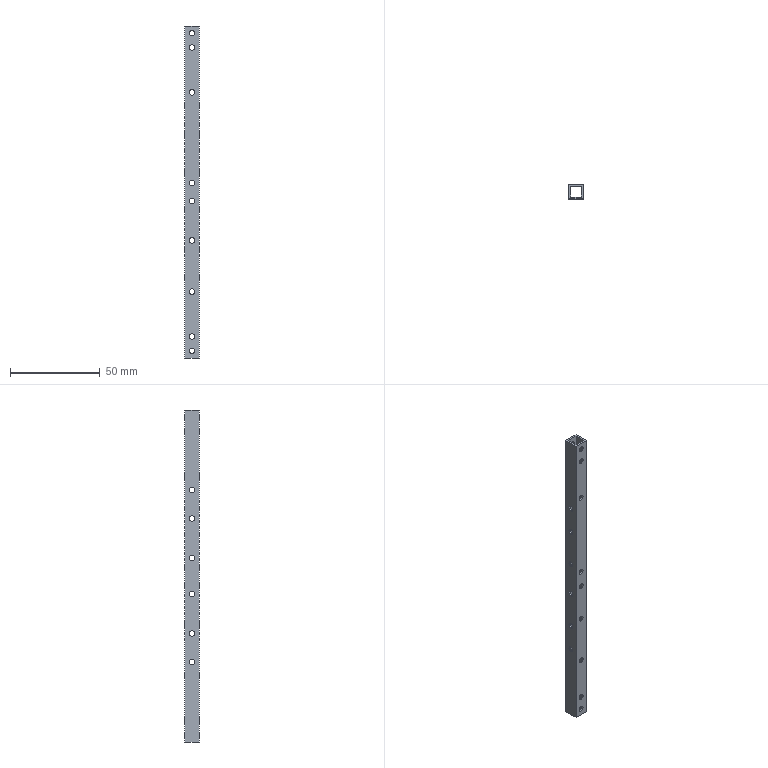Part | SolidWorks | features ICE 4, Extrusion 1 | 1 solid | 70 faces | box 8 x 8 x 185 mm | volume 4954 mm3 | cylinder 60 | plane 10 | commonest cylinder face diameters 3.1 x60